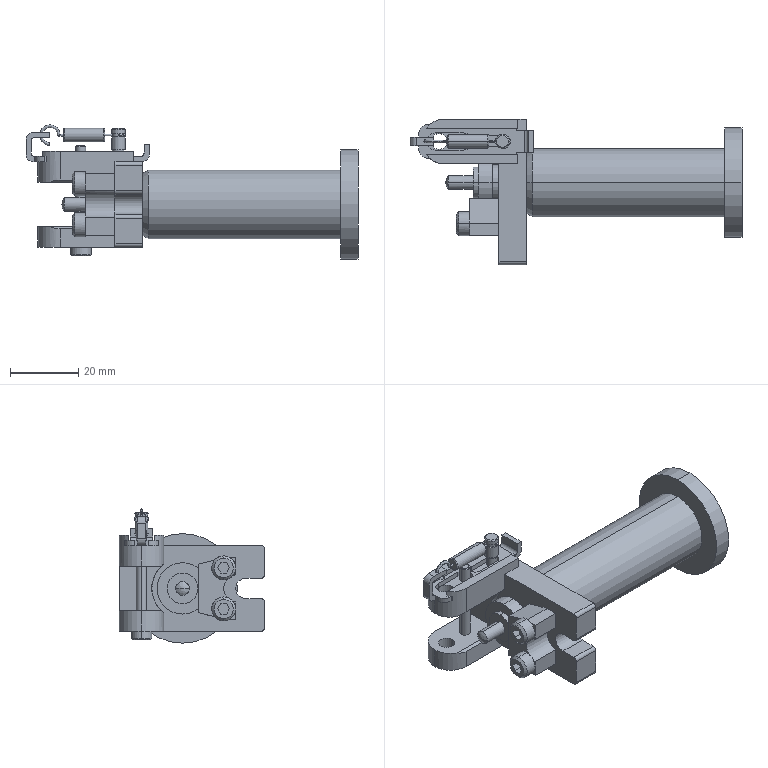Part | STEP file | 1105WWT2_2 | 1 solid | 208 faces | box 97 x 42.5 x 39.25 mm | volume 37426 mm3 | plane 100 | cylinder 78 | cone 16 | spline 14 | commonest cylinder face diameters 2 x9 4 x9 3 x6 6 x5 0.5 x4 4.7 x4